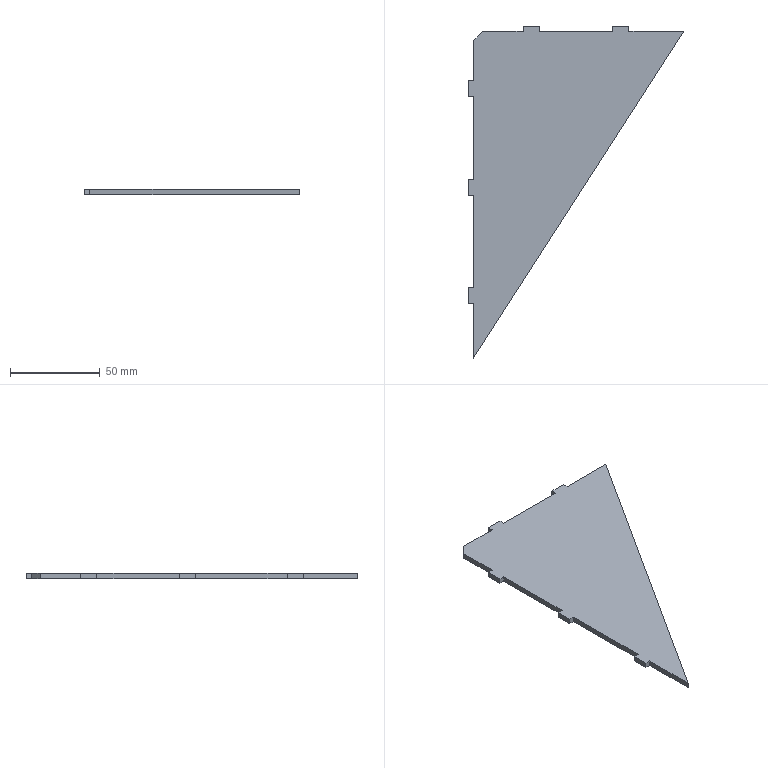Part | 1 solid | 26 faces | box 120 x 185 x 3 mm | volume 32309 mm3 | plane 26
STEP:
#1=CARTESIAN_POINT('',(0.,-36.5,-3.));
#2=VERTEX_POINT('',#1);
#3=CARTESIAN_POINT('',(0.,-82.5,-3.));
#4=VERTEX_POINT('',#3);
#5=CARTESIAN_POINT('',(0.,-182.,-3.));
#6=DIRECTION('',(0.,-1.,0.));
#7=VECTOR('',#6,1000.);
#8=LINE('',#5,#7);
#9=EDGE_CURVE('',#2,#4,#8,.T.);
#10=ORIENTED_EDGE('',*,*,#9,.T.);
#11=CARTESIAN_POINT('',(0.,-82.5,0.));
#12=VERTEX_POINT('',#11);
#13=CARTESIAN_POINT('',(0.,-82.5,0.));
#14=DIRECTION('',(0.,0.,-1.));
#15=VECTOR('',#14,1000.);
#16=LINE('',#13,#15);
#17=EDGE_CURVE('',#12,#4,#16,.T.);
#18=ORIENTED_EDGE('',*,*,#17,.F.);
#19=CARTESIAN_POINT('',(0.,-36.5,0.));
#20=VERTEX_POINT('',#19);
#21=CARTESIAN_POINT('',(0.,-182.,0.));
#22=DIRECTION('',(0.,-1.,0.));
#23=VECTOR('',#22,1000.);
#24=LINE('',#21,#23);
#25=EDGE_CURVE('',#20,#12,#24,.T.);
#26=ORIENTED_EDGE('',*,*,#25,.F.);
#27=CARTESIAN_POINT('',(0.,-36.5,-3.));
#28=DIRECTION('',(0.,0.,1.));
#29=VECTOR('',#28,1000.);
#30=LINE('',#27,#29);
#31=EDGE_CURVE('',#2,#20,#30,.T.);
#32=ORIENTED_EDGE('',*,*,#31,.F.);
#33=EDGE_LOOP('',(#10,#18,#26,#32));
#34=FACE_OUTER_BOUND('',#33,.T.);
#35=CARTESIAN_POINT('',(0.,-182.,-3.));
#36=DIRECTION('',(-1.,0.,0.));
#37=DIRECTION('',(0.,0.,1.));
#38=AXIS2_PLACEMENT_3D('',#35,#36,#37);
#39=PLANE('',#38);
#40=ADVANCED_FACE('',(#34),#39,.T.);
#41=CARTESIAN_POINT('',(0.,-91.5,0.));
#42=VERTEX_POINT('',#41);
#43=CARTESIAN_POINT('',(0.,-142.5,0.));
#44=VERTEX_POINT('',#43);
#45=CARTESIAN_POINT('',(0.,-182.,0.));
#46=DIRECTION('',(0.,-1.,0.));
#47=VECTOR('',#46,1000.);
#48=LINE('',#45,#47);
#49=EDGE_CURVE('',#42,#44,#48,.T.);
#50=ORIENTED_EDGE('',*,*,#49,.F.);
#51=CARTESIAN_POINT('',(0.,-91.5,-3.));
#52=VERTEX_POINT('',#51);
#53=CARTESIAN_POINT('',(0.,-91.5,0.));
#54=DIRECTION('',(0.,0.,1.));
#55=VECTOR('',#54,1000.);
#56=LINE('',#53,#55);
#57=EDGE_CURVE('',#52,#42,#56,.T.);
#58=ORIENTED_EDGE('',*,*,#57,.F.);
#59=CARTESIAN_POINT('',(0.,-142.5,-3.));
#60=VERTEX_POINT('',#59);
#61=CARTESIAN_POINT('',(0.,-182.,-3.));
#62=DIRECTION('',(0.,-1.,0.));
#63=VECTOR('',#62,1000.);
#64=LINE('',#61,#63);
#65=EDGE_CURVE('',#52,#60,#64,.T.);
#66=ORIENTED_EDGE('',*,*,#65,.T.);
#67=CARTESIAN_POINT('',(0.,-142.5,-3.));
#68=DIRECTION('',(0.,0.,-1.));
#69=VECTOR('',#68,1000.);
#70=LINE('',#67,#69);
#71=EDGE_CURVE('',#44,#60,#70,.T.);
#72=ORIENTED_EDGE('',*,*,#71,.F.);
#73=EDGE_LOOP('',(#50,#58,#66,#72));
#74=FACE_OUTER_BOUND('',#73,.T.);
#75=CARTESIAN_POINT('',(0.,-182.,-3.));
#76=DIRECTION('',(-1.,0.,0.));
#77=DIRECTION('',(0.,0.,1.));
#78=AXIS2_PLACEMENT_3D('',#75,#76,#77);
#79=PLANE('',#78);
#80=ADVANCED_FACE('',(#74),#79,.T.);
#81=CARTESIAN_POINT('',(0.,-5.,-3.));
#82=VERTEX_POINT('',#81);
#83=CARTESIAN_POINT('',(0.,-27.5,-3.));
#84=VERTEX_POINT('',#83);
#85=CARTESIAN_POINT('',(0.,-182.,-3.));
#86=DIRECTION('',(0.,-1.,0.));
#87=VECTOR('',#86,1000.);
#88=LINE('',#85,#87);
#89=EDGE_CURVE('',#82,#84,#88,.T.);
#90=ORIENTED_EDGE('',*,*,#89,.T.);
#91=CARTESIAN_POINT('',(0.,-27.5,0.));
#92=VERTEX_POINT('',#91);
#93=CARTESIAN_POINT('',(0.,-27.5,-3.));
#94=DIRECTION('',(0.,0.,-1.));
#95=VECTOR('',#94,1000.);
#96=LINE('',#93,#95);
#97=EDGE_CURVE('',#92,#84,#96,.T.);
#98=ORIENTED_EDGE('',*,*,#97,.F.);
#99=CARTESIAN_POINT('',(0.,-5.,0.));
#100=VERTEX_POINT('',#99);
#101=CARTESIAN_POINT('',(0.,-182.,0.));
#102=DIRECTION('',(0.,-1.,0.));
#103=VECTOR('',#102,1000.);
#104=LINE('',#101,#103);
#105=EDGE_CURVE('',#100,#92,#104,.T.);
#106=ORIENTED_EDGE('',*,*,#105,.F.);
#107=CARTESIAN_POINT('',(0.,-5.,-3.));
#108=DIRECTION('',(0.,0.,1.));
#109=VECTOR('',#108,1000.);
#110=LINE('',#107,#109);
#111=EDGE_CURVE('',#82,#100,#110,.T.);
#112=ORIENTED_EDGE('',*,*,#111,.F.);
#113=EDGE_LOOP('',(#90,#98,#106,#112));
#114=FACE_OUTER_BOUND('',#113,.T.);
#115=CARTESIAN_POINT('',(0.,-182.,-3.));
#116=DIRECTION('',(-1.,0.,0.));
#117=DIRECTION('',(0.,0.,1.));
#118=AXIS2_PLACEMENT_3D('',#115,#116,#117);
#119=PLANE('',#118);
#120=ADVANCED_FACE('',(#114),#119,.T.);
#121=CARTESIAN_POINT('',(77.5,0.,0.));
#122=VERTEX_POINT('',#121);
#123=CARTESIAN_POINT('',(36.5,0.,0.));
#124=VERTEX_POINT('',#123);
#125=CARTESIAN_POINT('',(5.,0.,0.));
#126=DIRECTION('',(-1.,0.,0.));
#127=VECTOR('',#126,1000.);
#128=LINE('',#125,#127);
#129=EDGE_CURVE('',#122,#124,#128,.T.);
#130=ORIENTED_EDGE('',*,*,#129,.F.);
#131=CARTESIAN_POINT('',(77.5,0.,-3.));
#132=VERTEX_POINT('',#131);
#133=CARTESIAN_POINT('',(77.5,0.,-3.));
#134=DIRECTION('',(0.,0.,1.));
#135=VECTOR('',#134,1000.);
#136=LINE('',#133,#135);
#137=EDGE_CURVE('',#132,#122,#136,.T.);
#138=ORIENTED_EDGE('',*,*,#137,.F.);
#139=CARTESIAN_POINT('',(36.5,0.,-3.));
#140=VERTEX_POINT('',#139);
#141=CARTESIAN_POINT('',(5.,0.,-3.));
#142=DIRECTION('',(-1.,0.,0.));
#143=VECTOR('',#142,1000.);
#144=LINE('',#141,#143);
#145=EDGE_CURVE('',#132,#140,#144,.T.);
#146=ORIENTED_EDGE('',*,*,#145,.T.);
#147=CARTESIAN_POINT('',(36.5,0.,-3.));
#148=DIRECTION('',(0.,0.,-1.));
#149=VECTOR('',#148,1000.);
#150=LINE('',#147,#149);
#151=EDGE_CURVE('',#124,#140,#150,.T.);
#152=ORIENTED_EDGE('',*,*,#151,.F.);
#153=EDGE_LOOP('',(#130,#138,#146,#152));
#154=FACE_OUTER_BOUND('',#153,.T.);
#155=CARTESIAN_POINT('',(5.,0.,-3.));
#156=DIRECTION('',(0.,1.,0.));
#157=DIRECTION('',(0.,0.,1.));
#158=AXIS2_PLACEMENT_3D('',#155,#156,#157);
#159=PLANE('',#158);
#160=ADVANCED_FACE('',(#154),#159,.T.);
#161=CARTESIAN_POINT('',(117.,0.,-3.));
#162=VERTEX_POINT('',#161);
#163=CARTESIAN_POINT('',(86.5,0.,-3.));
#164=VERTEX_POINT('',#163);
#165=CARTESIAN_POINT('',(5.,0.,-3.));
#166=DIRECTION('',(-1.,0.,0.));
#167=VECTOR('',#166,1000.);
#168=LINE('',#165,#167);
#169=EDGE_CURVE('',#162,#164,#168,.T.);
#170=ORIENTED_EDGE('',*,*,#169,.T.);
#171=CARTESIAN_POINT('',(86.5,0.,0.));
#172=VERTEX_POINT('',#171);
#173=CARTESIAN_POINT('',(86.5,0.,-3.));
#174=DIRECTION('',(0.,0.,-1.));
#175=VECTOR('',#174,1000.);
#176=LINE('',#173,#175);
#177=EDGE_CURVE('',#172,#164,#176,.T.);
#178=ORIENTED_EDGE('',*,*,#177,.F.);
#179=CARTESIAN_POINT('',(117.,0.,0.));
#180=VERTEX_POINT('',#179);
#181=CARTESIAN_POINT('',(5.,0.,0.));
#182=DIRECTION('',(-1.,0.,0.));
#183=VECTOR('',#182,1000.);
#184=LINE('',#181,#183);
#185=EDGE_CURVE('',#180,#172,#184,.T.);
#186=ORIENTED_EDGE('',*,*,#185,.F.);
#187=CARTESIAN_POINT('',(117.,0.,-3.));
#188=DIRECTION('',(0.,0.,1.));
#189=VECTOR('',#188,1000.);
#190=LINE('',#187,#189);
#191=EDGE_CURVE('',#162,#180,#190,.T.);
#192=ORIENTED_EDGE('',*,*,#191,.F.);
#193=EDGE_LOOP('',(#170,#178,#186,#192));
#194=FACE_OUTER_BOUND('',#193,.T.);
#195=CARTESIAN_POINT('',(5.,0.,-3.));
#196=DIRECTION('',(0.,1.,0.));
#197=DIRECTION('',(0.,0.,1.));
#198=AXIS2_PLACEMENT_3D('',#195,#196,#197);
#199=PLANE('',#198);
#200=ADVANCED_FACE('',(#194),#199,.T.);
#201=CARTESIAN_POINT('',(27.5,0.,-3.));
#202=VERTEX_POINT('',#201);
#203=CARTESIAN_POINT('',(27.5,0.,0.));
#204=VERTEX_POINT('',#203);
#205=CARTESIAN_POINT('',(27.5,0.,-3.));
#206=DIRECTION('',(0.,0.,1.));
#207=VECTOR('',#206,1000.);
#208=LINE('',#205,#207);
#209=EDGE_CURVE('',#202,#204,#208,.T.);
#210=ORIENTED_EDGE('',*,*,#209,.F.);
#211=CARTESIAN_POINT('',(5.,0.,-3.));
#212=VERTEX_POINT('',#211);
#213=CARTESIAN_POINT('',(5.,0.,-3.));
#214=DIRECTION('',(-1.,0.,0.));
#215=VECTOR('',#214,1000.);
#216=LINE('',#213,#215);
#217=EDGE_CURVE('',#202,#212,#216,.T.);
#218=ORIENTED_EDGE('',*,*,#217,.T.);
#219=CARTESIAN_POINT('',(5.,0.,0.));
#220=VERTEX_POINT('',#219);
#221=CARTESIAN_POINT('',(5.,0.,-3.));
#222=DIRECTION('',(0.,0.,1.));
#223=VECTOR('',#222,1000.);
#224=LINE('',#221,#223);
#225=EDGE_CURVE('',#212,#220,#224,.T.);
#226=ORIENTED_EDGE('',*,*,#225,.T.);
#227=CARTESIAN_POINT('',(5.,0.,0.));
#228=DIRECTION('',(-1.,0.,0.));
#229=VECTOR('',#228,1000.);
#230=LINE('',#227,#229);
#231=EDGE_CURVE('',#204,#220,#230,.T.);
#232=ORIENTED_EDGE('',*,*,#231,.F.);
#233=EDGE_LOOP('',(#210,#218,#226,#232));
#234=FACE_OUTER_BOUND('',#233,.T.);
#235=CARTESIAN_POINT('',(5.,0.,-3.));
#236=DIRECTION('',(0.,1.,0.));
#237=DIRECTION('',(0.,0.,1.));
#238=AXIS2_PLACEMENT_3D('',#235,#236,#237);
#239=PLANE('',#238);
#240=ADVANCED_FACE('',(#234),#239,.T.);
#241=CARTESIAN_POINT('',(0.,-182.,0.));
#242=VERTEX_POINT('',#241);
#243=CARTESIAN_POINT('',(117.,0.,0.));
#244=DIRECTION('',(0.5408,0.8412,0.));
#245=VECTOR('',#244,1000.);
#246=LINE('',#243,#245);
#247=EDGE_CURVE('',#242,#180,#246,.T.);
#248=ORIENTED_EDGE('',*,*,#247,.F.);
#249=CARTESIAN_POINT('',(0.,-182.,-3.));
#250=VERTEX_POINT('',#249);
#251=CARTESIAN_POINT('',(0.,-182.,-3.));
#252=DIRECTION('',(0.,0.,1.));
#253=VECTOR('',#252,1000.);
#254=LINE('',#251,#253);
#255=EDGE_CURVE('',#250,#242,#254,.T.);
#256=ORIENTED_EDGE('',*,*,#255,.F.);
#257=CARTESIAN_POINT('',(117.,0.,-3.));
#258=DIRECTION('',(0.5408,0.8412,0.));
#259=VECTOR('',#258,1000.);
#260=LINE('',#257,#259);
#261=EDGE_CURVE('',#250,#162,#260,.T.);
#262=ORIENTED_EDGE('',*,*,#261,.T.);
#263=ORIENTED_EDGE('',*,*,#191,.T.);
#264=EDGE_LOOP('',(#248,#256,#262,#263));
#265=FACE_OUTER_BOUND('',#264,.T.);
#266=CARTESIAN_POINT('',(117.,0.,-3.));
#267=DIRECTION('',(0.8412,-0.5408,0.));
#268=DIRECTION('',(0.5408,0.8412,0.));
#269=AXIS2_PLACEMENT_3D('',#266,#267,#268);
#270=PLANE('',#269);
#271=ADVANCED_FACE('',(#265),#270,.T.);
#272=CARTESIAN_POINT('',(0.,-151.5,-3.));
#273=VERTEX_POINT('',#272);
#274=CARTESIAN_POINT('',(0.,-151.5,0.));
#275=VERTEX_POINT('',#274);
#276=CARTESIAN_POINT('',(0.,-151.5,-3.));
#277=DIRECTION('',(0.,0.,1.));
#278=VECTOR('',#277,1000.);
#279=LINE('',#276,#278);
#280=EDGE_CURVE('',#273,#275,#279,.T.);
#281=ORIENTED_EDGE('',*,*,#280,.F.);
#282=CARTESIAN_POINT('',(0.,-182.,-3.));
#283=DIRECTION('',(0.,-1.,0.));
#284=VECTOR('',#283,1000.);
#285=LINE('',#282,#284);
#286=EDGE_CURVE('',#273,#250,#285,.T.);
#287=ORIENTED_EDGE('',*,*,#286,.T.);
#288=ORIENTED_EDGE('',*,*,#255,.T.);
#289=CARTESIAN_POINT('',(0.,-182.,0.));
#290=DIRECTION('',(0.,-1.,0.));
#291=VECTOR('',#290,1000.);
#292=LINE('',#289,#291);
#293=EDGE_CURVE('',#275,#242,#292,.T.);
#294=ORIENTED_EDGE('',*,*,#293,.F.);
#295=EDGE_LOOP('',(#281,#287,#288,#294));
#296=FACE_OUTER_BOUND('',#295,.T.);
#297=CARTESIAN_POINT('',(0.,-182.,-3.));
#298=DIRECTION('',(-1.,0.,0.));
#299=DIRECTION('',(0.,0.,1.));
#300=AXIS2_PLACEMENT_3D('',#297,#298,#299);
#301=PLANE('',#300);
#302=ADVANCED_FACE('',(#296),#301,.T.);
#303=CARTESIAN_POINT('',(5.,0.,0.));
#304=DIRECTION('',(-0.7071,-0.7071,0.));
#305=VECTOR('',#304,1000.);
#306=LINE('',#303,#305);
#307=EDGE_CURVE('',#220,#100,#306,.T.);
#308=ORIENTED_EDGE('',*,*,#307,.F.);
#309=ORIENTED_EDGE('',*,*,#225,.F.);
#310=CARTESIAN_POINT('',(5.,0.,-3.));
#311=DIRECTION('',(-0.7071,-0.7071,0.));
#312=VECTOR('',#311,1000.);
#313=LINE('',#310,#312);
#314=EDGE_CURVE('',#212,#82,#313,.T.);
#315=ORIENTED_EDGE('',*,*,#314,.T.);
#316=ORIENTED_EDGE('',*,*,#111,.T.);
#317=EDGE_LOOP('',(#308,#309,#315,#316));
#318=FACE_OUTER_BOUND('',#317,.T.);
#319=CARTESIAN_POINT('',(5.,0.,-3.));
#320=DIRECTION('',(-0.7071,0.7071,0.));
#321=DIRECTION('',(-0.7071,-0.7071,0.));
#322=AXIS2_PLACEMENT_3D('',#319,#320,#321);
#323=PLANE('',#322);
#324=ADVANCED_FACE('',(#318),#323,.T.);
#325=ORIENTED_EDGE('',*,*,#261,.F.);
#326=ORIENTED_EDGE('',*,*,#286,.F.);
#327=CARTESIAN_POINT('',(-3.,-151.5,-3.));
#328=VERTEX_POINT('',#327);
#329=CARTESIAN_POINT('',(-3.,-151.5,-3.));
#330=DIRECTION('',(1.,0.,0.));
#331=VECTOR('',#330,1000.);
#332=LINE('',#329,#331);
#333=EDGE_CURVE('',#328,#273,#332,.T.);
#334=ORIENTED_EDGE('',*,*,#333,.F.);
#335=CARTESIAN_POINT('',(-3.,-142.5,-3.));
#336=VERTEX_POINT('',#335);
#337=CARTESIAN_POINT('',(-3.,-142.5,-3.));
#338=DIRECTION('',(0.,-1.,0.));
#339=VECTOR('',#338,1000.);
#340=LINE('',#337,#339);
#341=EDGE_CURVE('',#336,#328,#340,.T.);
#342=ORIENTED_EDGE('',*,*,#341,.F.);
#343=CARTESIAN_POINT('',(-3.,-142.5,-3.));
#344=DIRECTION('',(1.,0.,0.));
#345=VECTOR('',#344,1000.);
#346=LINE('',#343,#345);
#347=EDGE_CURVE('',#336,#60,#346,.T.);
#348=ORIENTED_EDGE('',*,*,#347,.T.);
#349=ORIENTED_EDGE('',*,*,#65,.F.);
#350=CARTESIAN_POINT('',(-3.,-91.5,-3.));
#351=VERTEX_POINT('',#350);
#352=CARTESIAN_POINT('',(-3.,-91.5,-3.));
#353=DIRECTION('',(1.,0.,0.));
#354=VECTOR('',#353,1000.);
#355=LINE('',#352,#354);
#356=EDGE_CURVE('',#351,#52,#355,.T.);
#357=ORIENTED_EDGE('',*,*,#356,.F.);
#358=CARTESIAN_POINT('',(-3.,-82.5,-3.));
#359=VERTEX_POINT('',#358);
#360=CARTESIAN_POINT('',(-3.,-82.5,-3.));
#361=DIRECTION('',(0.,-1.,0.));
#362=VECTOR('',#361,1000.);
#363=LINE('',#360,#362);
#364=EDGE_CURVE('',#359,#351,#363,.T.);
#365=ORIENTED_EDGE('',*,*,#364,.F.);
#366=CARTESIAN_POINT('',(-3.,-82.5,-3.));
#367=DIRECTION('',(1.,0.,0.));
#368=VECTOR('',#367,1000.);
#369=LINE('',#366,#368);
#370=EDGE_CURVE('',#359,#4,#369,.T.);
#371=ORIENTED_EDGE('',*,*,#370,.T.);
#372=ORIENTED_EDGE('',*,*,#9,.F.);
#373=CARTESIAN_POINT('',(-3.,-36.5,-3.));
#374=VERTEX_POINT('',#373);
#375=CARTESIAN_POINT('',(-3.,-36.5,-3.));
#376=DIRECTION('',(1.,0.,0.));
#377=VECTOR('',#376,1000.);
#378=LINE('',#375,#377);
#379=EDGE_CURVE('',#374,#2,#378,.T.);
#380=ORIENTED_EDGE('',*,*,#379,.F.);
#381=CARTESIAN_POINT('',(-3.,-27.5,-3.));
#382=VERTEX_POINT('',#381);
#383=CARTESIAN_POINT('',(-3.,-27.5,-3.));
#384=DIRECTION('',(0.,-1.,0.));
#385=VECTOR('',#384,1000.);
#386=LINE('',#383,#385);
#387=EDGE_CURVE('',#382,#374,#386,.T.);
#388=ORIENTED_EDGE('',*,*,#387,.F.);
#389=CARTESIAN_POINT('',(-3.,-27.5,-3.));
#390=DIRECTION('',(1.,0.,0.));
#391=VECTOR('',#390,1000.);
#392=LINE('',#389,#391);
#393=EDGE_CURVE('',#382,#84,#392,.T.);
#394=ORIENTED_EDGE('',*,*,#393,.T.);
#395=ORIENTED_EDGE('',*,*,#89,.F.);
#396=ORIENTED_EDGE('',*,*,#314,.F.);
#397=ORIENTED_EDGE('',*,*,#217,.F.);
#398=CARTESIAN_POINT('',(27.5,3.,-3.));
#399=VERTEX_POINT('',#398);
#400=CARTESIAN_POINT('',(27.5,3.,-3.));
#401=DIRECTION('',(0.,-1.,0.));
#402=VECTOR('',#401,1000.);
#403=LINE('',#400,#402);
#404=EDGE_CURVE('',#399,#202,#403,.T.);
#405=ORIENTED_EDGE('',*,*,#404,.F.);
#406=CARTESIAN_POINT('',(36.5,3.,-3.));
#407=VERTEX_POINT('',#406);
#408=CARTESIAN_POINT('',(27.5,3.,-3.));
#409=DIRECTION('',(-1.,0.,0.));
#410=VECTOR('',#409,1000.);
#411=LINE('',#408,#410);
#412=EDGE_CURVE('',#407,#399,#411,.T.);
#413=ORIENTED_EDGE('',*,*,#412,.F.);
#414=CARTESIAN_POINT('',(36.5,3.,-3.));
#415=DIRECTION('',(0.,-1.,0.));
#416=VECTOR('',#415,1000.);
#417=LINE('',#414,#416);
#418=EDGE_CURVE('',#407,#140,#417,.T.);
#419=ORIENTED_EDGE('',*,*,#418,.T.);
#420=ORIENTED_EDGE('',*,*,#145,.F.);
#421=CARTESIAN_POINT('',(77.5,3.,-3.));
#422=VERTEX_POINT('',#421);
#423=CARTESIAN_POINT('',(77.5,3.,-3.));
#424=DIRECTION('',(0.,-1.,0.));
#425=VECTOR('',#424,1000.);
#426=LINE('',#423,#425);
#427=EDGE_CURVE('',#422,#132,#426,.T.);
#428=ORIENTED_EDGE('',*,*,#427,.F.);
#429=CARTESIAN_POINT('',(86.5,3.,-3.));
#430=VERTEX_POINT('',#429);
#431=CARTESIAN_POINT('',(77.5,3.,-3.));
#432=DIRECTION('',(-1.,0.,0.));
#433=VECTOR('',#432,1000.);
#434=LINE('',#431,#433);
#435=EDGE_CURVE('',#430,#422,#434,.T.);
#436=ORIENTED_EDGE('',*,*,#435,.F.);
#437=CARTESIAN_POINT('',(86.5,3.,-3.));
#438=DIRECTION('',(0.,-1.,0.));
#439=VECTOR('',#438,1000.);
#440=LINE('',#437,#439);
#441=EDGE_CURVE('',#430,#164,#440,.T.);
#442=ORIENTED_EDGE('',*,*,#441,.T.);
#443=ORIENTED_EDGE('',*,*,#169,.F.);
#444=EDGE_LOOP('',(#325,#326,#334,#342,#348,#349,#357,#365,#371,#372,#380,#388,#394,#395,#396,#397,#405,#413,#419,#420,#428,#436,#442,#443));
#445=FACE_OUTER_BOUND('',#444,.T.);
#446=CARTESIAN_POINT('',(0.,0.,-3.));
#447=DIRECTION('',(0.,0.,1.));
#448=DIRECTION('',(1.,0.,0.));
#449=AXIS2_PLACEMENT_3D('',#446,#447,#448);
#450=PLANE('',#449);
#451=ADVANCED_FACE('',(#445),#450,.F.);
#452=ORIENTED_EDGE('',*,*,#247,.T.);
#453=ORIENTED_EDGE('',*,*,#185,.T.);
#454=CARTESIAN_POINT('',(86.5,3.,0.));
#455=VERTEX_POINT('',#454);
#456=CARTESIAN_POINT('',(86.5,3.,0.));
#457=DIRECTION('',(0.,-1.,0.));
#458=VECTOR('',#457,1000.);
#459=LINE('',#456,#458);
#460=EDGE_CURVE('',#455,#172,#459,.T.);
#461=ORIENTED_EDGE('',*,*,#460,.F.);
#462=CARTESIAN_POINT('',(77.5,3.,0.));
#463=VERTEX_POINT('',#462);
#464=CARTESIAN_POINT('',(77.5,3.,0.));
#465=DIRECTION('',(1.,0.,0.));
#466=VECTOR('',#465,1000.);
#467=LINE('',#464,#466);
#468=EDGE_CURVE('',#463,#455,#467,.T.);
#469=ORIENTED_EDGE('',*,*,#468,.F.);
#470=CARTESIAN_POINT('',(77.5,3.,0.));
#471=DIRECTION('',(0.,-1.,0.));
#472=VECTOR('',#471,1000.);
#473=LINE('',#470,#472);
#474=EDGE_CURVE('',#463,#122,#473,.T.);
#475=ORIENTED_EDGE('',*,*,#474,.T.);
#476=ORIENTED_EDGE('',*,*,#129,.T.);
#477=CARTESIAN_POINT('',(36.5,3.,0.));
#478=VERTEX_POINT('',#477);
#479=CARTESIAN_POINT('',(36.5,3.,0.));
#480=DIRECTION('',(0.,-1.,0.));
#481=VECTOR('',#480,1000.);
#482=LINE('',#479,#481);
#483=EDGE_CURVE('',#478,#124,#482,.T.);
#484=ORIENTED_EDGE('',*,*,#483,.F.);
#485=CARTESIAN_POINT('',(27.5,3.,0.));
#486=VERTEX_POINT('',#485);
#487=CARTESIAN_POINT('',(27.5,3.,0.));
#488=DIRECTION('',(1.,0.,0.));
#489=VECTOR('',#488,1000.);
#490=LINE('',#487,#489);
#491=EDGE_CURVE('',#486,#478,#490,.T.);
#492=ORIENTED_EDGE('',*,*,#491,.F.);
#493=CARTESIAN_POINT('',(27.5,3.,0.));
#494=DIRECTION('',(0.,-1.,0.));
#495=VECTOR('',#494,1000.);
#496=LINE('',#493,#495);
#497=EDGE_CURVE('',#486,#204,#496,.T.);
#498=ORIENTED_EDGE('',*,*,#497,.T.);
#499=ORIENTED_EDGE('',*,*,#231,.T.);
#500=ORIENTED_EDGE('',*,*,#307,.T.);
#501=ORIENTED_EDGE('',*,*,#105,.T.);
#502=CARTESIAN_POINT('',(-3.,-27.5,0.));
#503=VERTEX_POINT('',#502);
#504=CARTESIAN_POINT('',(-3.,-27.5,0.));
#505=DIRECTION('',(1.,0.,0.));
#506=VECTOR('',#505,1000.);
#507=LINE('',#504,#506);
#508=EDGE_CURVE('',#503,#92,#507,.T.);
#509=ORIENTED_EDGE('',*,*,#508,.F.);
#510=CARTESIAN_POINT('',(-3.,-36.5,0.));
#511=VERTEX_POINT('',#510);
#512=CARTESIAN_POINT('',(-3.,-27.5,0.));
#513=DIRECTION('',(0.,1.,0.));
#514=VECTOR('',#513,1000.);
#515=LINE('',#512,#514);
#516=EDGE_CURVE('',#511,#503,#515,.T.);
#517=ORIENTED_EDGE('',*,*,#516,.F.);
#518=CARTESIAN_POINT('',(-3.,-36.5,0.));
#519=DIRECTION('',(1.,0.,0.));
#520=VECTOR('',#519,1000.);
#521=LINE('',#518,#520);
#522=EDGE_CURVE('',#511,#20,#521,.T.);
#523=ORIENTED_EDGE('',*,*,#522,.T.);
#524=ORIENTED_EDGE('',*,*,#25,.T.);
#525=CARTESIAN_POINT('',(-3.,-82.5,0.));
#526=VERTEX_POINT('',#525);
#527=CARTESIAN_POINT('',(-3.,-82.5,0.));
#528=DIRECTION('',(1.,0.,0.));
#529=VECTOR('',#528,1000.);
#530=LINE('',#527,#529);
#531=EDGE_CURVE('',#526,#12,#530,.T.);
#532=ORIENTED_EDGE('',*,*,#531,.F.);
#533=CARTESIAN_POINT('',(-3.,-91.5,0.));
#534=VERTEX_POINT('',#533);
#535=CARTESIAN_POINT('',(-3.,-82.5,0.));
#536=DIRECTION('',(0.,1.,0.));
#537=VECTOR('',#536,1000.);
#538=LINE('',#535,#537);
#539=EDGE_CURVE('',#534,#526,#538,.T.);
#540=ORIENTED_EDGE('',*,*,#539,.F.);
#541=CARTESIAN_POINT('',(-3.,-91.5,0.));
#542=DIRECTION('',(1.,0.,0.));
#543=VECTOR('',#542,1000.);
#544=LINE('',#541,#543);
#545=EDGE_CURVE('',#534,#42,#544,.T.);
#546=ORIENTED_EDGE('',*,*,#545,.T.);
#547=ORIENTED_EDGE('',*,*,#49,.T.);
#548=CARTESIAN_POINT('',(-3.,-142.5,0.));
#549=VERTEX_POINT('',#548);
#550=CARTESIAN_POINT('',(-3.,-142.5,0.));
#551=DIRECTION('',(1.,0.,0.));
#552=VECTOR('',#551,1000.);
#553=LINE('',#550,#552);
#554=EDGE_CURVE('',#549,#44,#553,.T.);
#555=ORIENTED_EDGE('',*,*,#554,.F.);
#556=CARTESIAN_POINT('',(-3.,-151.5,0.));
#557=VERTEX_POINT('',#556);
#558=CARTESIAN_POINT('',(-3.,-142.5,0.));
#559=DIRECTION('',(0.,1.,0.));
#560=VECTOR('',#559,1000.);
#561=LINE('',#558,#560);
#562=EDGE_CURVE('',#557,#549,#561,.T.);
#563=ORIENTED_EDGE('',*,*,#562,.F.);
#564=CARTESIAN_POINT('',(-3.,-151.5,0.));
#565=DIRECTION('',(1.,0.,0.));
#566=VECTOR('',#565,1000.);
#567=LINE('',#564,#566);
#568=EDGE_CURVE('',#557,#275,#567,.T.);
#569=ORIENTED_EDGE('',*,*,#568,.T.);
#570=ORIENTED_EDGE('',*,*,#293,.T.);
#571=EDGE_LOOP('',(#452,#453,#461,#469,#475,#476,#484,#492,#498,#499,#500,#501,#509,#517,#523,#524,#532,#540,#546,#547,#555,#563,#569,#570));
#572=FACE_OUTER_BOUND('',#571,.T.);
#573=CARTESIAN_POINT('',(0.,0.,0.));
#574=DIRECTION('',(0.,0.,1.));
#575=DIRECTION('',(1.,0.,0.));
#576=AXIS2_PLACEMENT_3D('',#573,#574,#575);
#577=PLANE('',#576);
#578=ADVANCED_FACE('',(#572),#577,.T.);
#579=ORIENTED_EDGE('',*,*,#209,.T.);
#580=ORIENTED_EDGE('',*,*,#497,.F.);
#581=CARTESIAN_POINT('',(27.5,3.,-3.));
#582=DIRECTION('',(0.,0.,1.));
#583=VECTOR('',#582,1000.);
#584=LINE('',#581,#583);
#585=EDGE_CURVE('',#399,#486,#584,.T.);
#586=ORIENTED_EDGE('',*,*,#585,.F.);
#587=ORIENTED_EDGE('',*,*,#404,.T.);
#588=EDGE_LOOP('',(#579,#580,#586,#587));
#589=FACE_OUTER_BOUND('',#588,.T.);
#590=CARTESIAN_POINT('',(27.5,3.,-3.));
#591=DIRECTION('',(1.,0.,0.));
#592=DIRECTION('',(0.,0.,-1.));
#593=AXIS2_PLACEMENT_3D('',#590,#591,#592);
#594=PLANE('',#593);
#595=ADVANCED_FACE('',(#589),#594,.F.);
#596=ORIENTED_EDGE('',*,*,#151,.T.);
#597=ORIENTED_EDGE('',*,*,#418,.F.);
#598=CARTESIAN_POINT('',(36.5,3.,-3.));
#599=DIRECTION('',(0.,0.,-1.));
#600=VECTOR('',#599,1000.);
#601=LINE('',#598,#600);
#602=EDGE_CURVE('',#478,#407,#601,.T.);
#603=ORIENTED_EDGE('',*,*,#602,.F.);
#604=ORIENTED_EDGE('',*,*,#483,.T.);
#605=EDGE_LOOP('',(#596,#597,#603,#604));
#606=FACE_OUTER_BOUND('',#605,.T.);
#607=CARTESIAN_POINT('',(36.5,3.,-3.));
#608=DIRECTION('',(-1.,0.,0.));
#609=DIRECTION('',(0.,0.,1.));
#610=AXIS2_PLACEMENT_3D('',#607,#608,#609);
#611=PLANE('',#610);
#612=ADVANCED_FACE('',(#606),#611,.F.);
#613=ORIENTED_EDGE('',*,*,#585,.T.);
#614=ORIENTED_EDGE('',*,*,#491,.T.);
#615=ORIENTED_EDGE('',*,*,#602,.T.);
#616=ORIENTED_EDGE('',*,*,#412,.T.);
#617=EDGE_LOOP('',(#613,#614,#615,#616));
#618=FACE_OUTER_BOUND('',#617,.T.);
#619=CARTESIAN_POINT('',(0.,3.,0.));
#620=DIRECTION('',(0.,1.,0.));
#621=DIRECTION('',(0.,0.,1.));
#622=AXIS2_PLACEMENT_3D('',#619,#620,#621);
#623=PLANE('',#622);
#624=ADVANCED_FACE('',(#618),#623,.T.);
#625=ORIENTED_EDGE('',*,*,#137,.T.);
#626=ORIENTED_EDGE('',*,*,#474,.F.);
#627=CARTESIAN_POINT('',(77.5,3.,-3.));
#628=DIRECTION('',(0.,0.,1.));
#629=VECTOR('',#628,1000.);
#630=LINE('',#627,#629);
#631=EDGE_CURVE('',#422,#463,#630,.T.);
#632=ORIENTED_EDGE('',*,*,#631,.F.);
#633=ORIENTED_EDGE('',*,*,#427,.T.);
#634=EDGE_LOOP('',(#625,#626,#632,#633));
#635=FACE_OUTER_BOUND('',#634,.T.);
#636=CARTESIAN_POINT('',(77.5,3.,-3.));
#637=DIRECTION('',(1.,0.,0.));
#638=DIRECTION('',(0.,0.,-1.));
#639=AXIS2_PLACEMENT_3D('',#636,#637,#638);
#640=PLANE('',#639);
#641=ADVANCED_FACE('',(#635),#640,.F.);
#642=ORIENTED_EDGE('',*,*,#177,.T.);
#643=ORIENTED_EDGE('',*,*,#441,.F.);
#644=CARTESIAN_POINT('',(86.5,3.,-3.));
#645=DIRECTION('',(0.,0.,-1.));
#646=VECTOR('',#645,1000.);
#647=LINE('',#644,#646);
#648=EDGE_CURVE('',#455,#430,#647,.T.);
#649=ORIENTED_EDGE('',*,*,#648,.F.);
#650=ORIENTED_EDGE('',*,*,#460,.T.);
#651=EDGE_LOOP('',(#642,#643,#649,#650));
#652=FACE_OUTER_BOUND('',#651,.T.);
#653=CARTESIAN_POINT('',(86.5,3.,-3.));
#654=DIRECTION('',(-1.,0.,0.));
#655=DIRECTION('',(0.,0.,1.));
#656=AXIS2_PLACEMENT_3D('',#653,#654,#655);
#657=PLANE('',#656);
#658=ADVANCED_FACE('',(#652),#657,.F.);
#659=ORIENTED_EDGE('',*,*,#631,.T.);
#660=ORIENTED_EDGE('',*,*,#468,.T.);
#661=ORIENTED_EDGE('',*,*,#648,.T.);
#662=ORIENTED_EDGE('',*,*,#435,.T.);
#663=EDGE_LOOP('',(#659,#660,#661,#662));
#664=FACE_OUTER_BOUND('',#663,.T.);
#665=CARTESIAN_POINT('',(0.,3.,0.));
#666=DIRECTION('',(0.,1.,0.));
#667=DIRECTION('',(0.,0.,1.));
#668=AXIS2_PLACEMENT_3D('',#665,#666,#667);
#669=PLANE('',#668);
#670=ADVANCED_FACE('',(#664),#669,.T.);
#671=ORIENTED_EDGE('',*,*,#280,.T.);
#672=ORIENTED_EDGE('',*,*,#568,.F.);
#673=CARTESIAN_POINT('',(-3.,-151.5,-3.));
#674=DIRECTION('',(0.,0.,1.));
#675=VECTOR('',#674,1000.);
#676=LINE('',#673,#675);
#677=EDGE_CURVE('',#328,#557,#676,.T.);
#678=ORIENTED_EDGE('',*,*,#677,.F.);
#679=ORIENTED_EDGE('',*,*,#333,.T.);
#680=EDGE_LOOP('',(#671,#672,#678,#679));
#681=FACE_OUTER_BOUND('',#680,.T.);
#682=CARTESIAN_POINT('',(-3.,-151.5,-3.));
#683=DIRECTION('',(0.,1.,0.));
#684=DIRECTION('',(0.,0.,1.));
#685=AXIS2_PLACEMENT_3D('',#682,#683,#684);
#686=PLANE('',#685);
#687=ADVANCED_FACE('',(#681),#686,.F.);
#688=ORIENTED_EDGE('',*,*,#71,.T.);
#689=ORIENTED_EDGE('',*,*,#347,.F.);
#690=CARTESIAN_POINT('',(-3.,-142.5,-3.));
#691=DIRECTION('',(0.,0.,-1.));
#692=VECTOR('',#691,1000.);
#693=LINE('',#690,#692);
#694=EDGE_CURVE('',#549,#336,#693,.T.);
#695=ORIENTED_EDGE('',*,*,#694,.F.);
#696=ORIENTED_EDGE('',*,*,#554,.T.);
#697=EDGE_LOOP('',(#688,#689,#695,#696));
#698=FACE_OUTER_BOUND('',#697,.T.);
#699=CARTESIAN_POINT('',(-3.,-142.5,-3.));
#700=DIRECTION('',(0.,-1.,0.));
#701=DIRECTION('',(0.,0.,-1.));
#702=AXIS2_PLACEMENT_3D('',#699,#700,#701);
#703=PLANE('',#702);
#704=ADVANCED_FACE('',(#698),#703,.F.);
#705=ORIENTED_EDGE('',*,*,#341,.T.);
#706=ORIENTED_EDGE('',*,*,#677,.T.);
#707=ORIENTED_EDGE('',*,*,#562,.T.);
#708=ORIENTED_EDGE('',*,*,#694,.T.);
#709=EDGE_LOOP('',(#705,#706,#707,#708));
#710=FACE_OUTER_BOUND('',#709,.T.);
#711=CARTESIAN_POINT('',(-3.,0.,0.));
#712=DIRECTION('',(-1.,0.,0.));
#713=DIRECTION('',(0.,0.,1.));
#714=AXIS2_PLACEMENT_3D('',#711,#712,#713);
#715=PLANE('',#714);
#716=ADVANCED_FACE('',(#710),#715,.T.);
#717=ORIENTED_EDGE('',*,*,#31,.T.);
#718=ORIENTED_EDGE('',*,*,#522,.F.);
#719=CARTESIAN_POINT('',(-3.,-36.5,-3.));
#720=DIRECTION('',(0.,0.,1.));
#721=VECTOR('',#720,1000.);
#722=LINE('',#719,#721);
#723=EDGE_CURVE('',#374,#511,#722,.T.);
#724=ORIENTED_EDGE('',*,*,#723,.F.);
#725=ORIENTED_EDGE('',*,*,#379,.T.);
#726=EDGE_LOOP('',(#717,#718,#724,#725));
#727=FACE_OUTER_BOUND('',#726,.T.);
#728=CARTESIAN_POINT('',(-3.,-36.5,-3.));
#729=DIRECTION('',(0.,1.,0.));
#730=DIRECTION('',(0.,0.,1.));
#731=AXIS2_PLACEMENT_3D('',#728,#729,#730);
#732=PLANE('',#731);
#733=ADVANCED_FACE('',(#727),#732,.F.);
#734=ORIENTED_EDGE('',*,*,#97,.T.);
#735=ORIENTED_EDGE('',*,*,#393,.F.);
#736=CARTESIAN_POINT('',(-3.,-27.5,-3.));
#737=DIRECTION('',(0.,0.,-1.));
#738=VECTOR('',#737,1000.);
#739=LINE('',#736,#738);
#740=EDGE_CURVE('',#503,#382,#739,.T.);
#741=ORIENTED_EDGE('',*,*,#740,.F.);
#742=ORIENTED_EDGE('',*,*,#508,.T.);
#743=EDGE_LOOP('',(#734,#735,#741,#742));
#744=FACE_OUTER_BOUND('',#743,.T.);
#745=CARTESIAN_POINT('',(-3.,-27.5,-3.));
#746=DIRECTION('',(0.,-1.,0.));
#747=DIRECTION('',(0.,0.,-1.));
#748=AXIS2_PLACEMENT_3D('',#745,#746,#747);
#749=PLANE('',#748);
#750=ADVANCED_FACE('',(#744),#749,.F.);
#751=ORIENTED_EDGE('',*,*,#387,.T.);
#752=ORIENTED_EDGE('',*,*,#723,.T.);
#753=ORIENTED_EDGE('',*,*,#516,.T.);
#754=ORIENTED_EDGE('',*,*,#740,.T.);
#755=EDGE_LOOP('',(#751,#752,#753,#754));
#756=FACE_OUTER_BOUND('',#755,.T.);
#757=CARTESIAN_POINT('',(-3.,0.,0.));
#758=DIRECTION('',(-1.,0.,0.));
#759=DIRECTION('',(0.,0.,1.));
#760=AXIS2_PLACEMENT_3D('',#757,#758,#759);
#761=PLANE('',#760);
#762=ADVANCED_FACE('',(#756),#761,.T.);
#763=ORIENTED_EDGE('',*,*,#17,.T.);
#764=ORIENTED_EDGE('',*,*,#370,.F.);
#765=CARTESIAN_POINT('',(-3.,-82.5,0.));
#766=DIRECTION('',(0.,0.,-1.));
#767=VECTOR('',#766,1000.);
#768=LINE('',#765,#767);
#769=EDGE_CURVE('',#526,#359,#768,.T.);
#770=ORIENTED_EDGE('',*,*,#769,.F.);
#771=ORIENTED_EDGE('',*,*,#531,.T.);
#772=EDGE_LOOP('',(#763,#764,#770,#771));
#773=FACE_OUTER_BOUND('',#772,.T.);
#774=CARTESIAN_POINT('',(-3.,-82.5,0.));
#775=DIRECTION('',(0.,-1.,0.));
#776=DIRECTION('',(0.,0.,-1.));
#777=AXIS2_PLACEMENT_3D('',#774,#775,#776);
#778=PLANE('',#777);
#779=ADVANCED_FACE('',(#773),#778,.F.);
#780=ORIENTED_EDGE('',*,*,#57,.T.);
#781=ORIENTED_EDGE('',*,*,#545,.F.);
#782=CARTESIAN_POINT('',(-3.,-91.5,0.));
#783=DIRECTION('',(0.,0.,1.));
#784=VECTOR('',#783,1000.);
#785=LINE('',#782,#784);
#786=EDGE_CURVE('',#351,#534,#785,.T.);
#787=ORIENTED_EDGE('',*,*,#786,.F.);
#788=ORIENTED_EDGE('',*,*,#356,.T.);
#789=EDGE_LOOP('',(#780,#781,#787,#788));
#790=FACE_OUTER_BOUND('',#789,.T.);
#791=CARTESIAN_POINT('',(-3.,-91.5,0.));
#792=DIRECTION('',(0.,1.,0.));
#793=DIRECTION('',(0.,0.,1.));
#794=AXIS2_PLACEMENT_3D('',#791,#792,#793);
#795=PLANE('',#794);
#796=ADVANCED_FACE('',(#790),#795,.F.);
#797=ORIENTED_EDGE('',*,*,#539,.T.);
#798=ORIENTED_EDGE('',*,*,#769,.T.);
#799=ORIENTED_EDGE('',*,*,#364,.T.);
#800=ORIENTED_EDGE('',*,*,#786,.T.);
#801=EDGE_LOOP('',(#797,#798,#799,#800));
#802=FACE_OUTER_BOUND('',#801,.T.);
#803=CARTESIAN_POINT('',(-3.,0.,0.));
#804=DIRECTION('',(1.,0.,0.));
#805=DIRECTION('',(0.,0.,-1.));
#806=AXIS2_PLACEMENT_3D('',#803,#804,#805);
#807=PLANE('',#806);
#808=ADVANCED_FACE('',(#802),#807,.F.);
#809=CLOSED_SHELL('',(#40,#80,#120,#160,#200,#240,#271,#302,#324,#451,#578,#595,#612,#624,#641,#658,#670,#687,#704,#716,#733,#750,#762,#779,#796,#808));
#810=MANIFOLD_SOLID_BREP('',#809);
#811=CARTESIAN_POINT('',(0.,0.,0.));
#812=DIRECTION('',(0.,0.,1.));
#813=DIRECTION('',(1.,0.,0.));
#814=AXIS2_PLACEMENT_3D('',#811,#812,#813);
#815=(LENGTH_UNIT()NAMED_UNIT(*)SI_UNIT(.MILLI.,.METRE.));
#816=UNCERTAINTY_MEASURE_WITH_UNIT(LENGTH_MEASURE(0.00001),#815,'','');
#817=(NAMED_UNIT(*)PLANE_ANGLE_UNIT()SI_UNIT($,.RADIAN.));
#818=(NAMED_UNIT(*)SI_UNIT($,.STERADIAN.)SOLID_ANGLE_UNIT());
#819=(GEOMETRIC_REPRESENTATION_CONTEXT(3)GLOBAL_UNCERTAINTY_ASSIGNED_CONTEXT((#816))GLOBAL_UNIT_ASSIGNED_CONTEXT((#815,#817,#818))REPRESENTATION_CONTEXT('',''));
#820=ADVANCED_BREP_SHAPE_REPRESENTATION('',(#810,#814),#819);